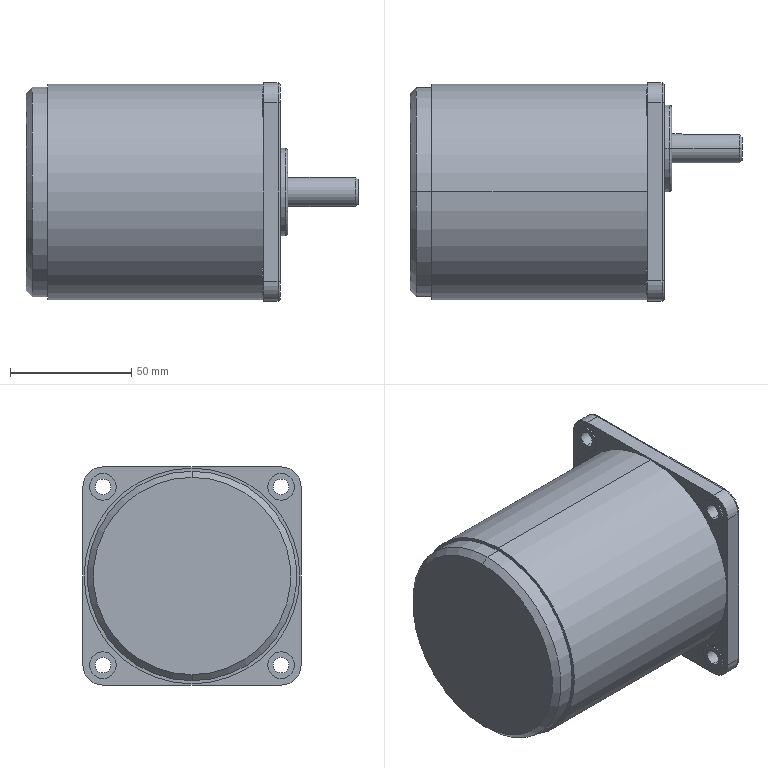Part | STEP file | 0228_101_Motor_5RK40GN-C | 1 solid | 61 faces | box 137 x 90 x 90 mm | volume 667092 mm3 | cylinder 33 | plane 17 | torus 6 | cone 5 | commonest cylinder face diameters 6.5 x8 11 x8 2 x4 16.4 x4 12 x2 36 x2